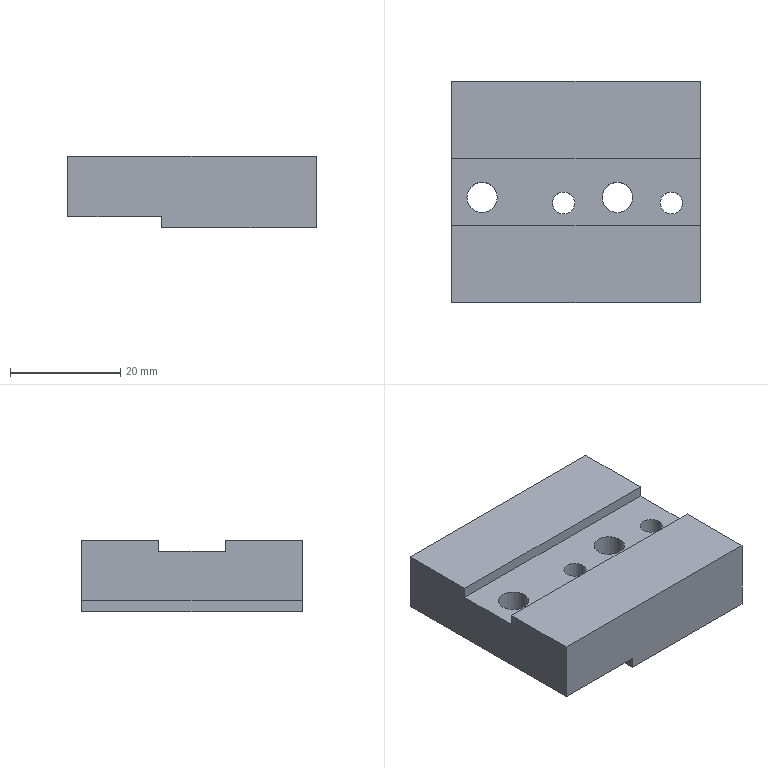Part | NX | features BREP 1 | 1 solid | 42 faces | box 45 x 40 x 13 mm | volume 19304 mm3 | cylinder 20 | plane 14 | cone 8 | commonest cylinder face diameters 3.3 x8 4 x4 5.5 x4 10 x4
STEP:
#1=CARTESIAN_POINT('',(-698.312,30.27,5.));
#2=VERTEX_POINT('',#1);
#3=CARTESIAN_POINT('',(-708.312,30.27,5.));
#4=VERTEX_POINT('',#3);
#5=CARTESIAN_POINT('',(-703.312,30.27,5.));
#6=DIRECTION('',(0.,0.,-1.));
#7=DIRECTION('',(-1.,0.,0.));
#8=AXIS2_PLACEMENT_3D('',#5,#6,#7);
#9=CIRCLE('',#8,5.);
#10=EDGE_CURVE('',#2,#4,#9,.T.);
#11=ORIENTED_EDGE('',*,*,#10,.F.);
#12=CARTESIAN_POINT('',(-698.312,30.27,0.));
#13=VERTEX_POINT('',#12);
#14=CARTESIAN_POINT('',(-698.312,30.27,0.));
#15=DIRECTION('',(0.,0.,-1.));
#16=VECTOR('',#15,1000.);
#17=LINE('',#14,#16);
#18=EDGE_CURVE('',#2,#13,#17,.T.);
#19=ORIENTED_EDGE('',*,*,#18,.T.);
#20=CARTESIAN_POINT('',(-708.312,30.27,0.));
#21=VERTEX_POINT('',#20);
#22=CARTESIAN_POINT('',(-703.312,30.27,0.));
#23=DIRECTION('',(0.,0.,-1.));
#24=DIRECTION('',(-1.,0.,0.));
#25=AXIS2_PLACEMENT_3D('',#22,#23,#24);
#26=CIRCLE('',#25,5.);
#27=EDGE_CURVE('',#13,#21,#26,.T.);
#28=ORIENTED_EDGE('',*,*,#27,.T.);
#29=CARTESIAN_POINT('',(-708.312,30.27,0.));
#30=DIRECTION('',(0.,0.,-1.));
#31=VECTOR('',#30,1000.);
#32=LINE('',#29,#31);
#33=EDGE_CURVE('',#4,#21,#32,.T.);
#34=ORIENTED_EDGE('',*,*,#33,.F.);
#35=EDGE_LOOP('',(#11,#19,#28,#34));
#36=FACE_BOUND('',#35,.T.);
#37=CARTESIAN_POINT('',(-703.312,30.27,0.));
#38=DIRECTION('',(0.,0.,-1.));
#39=DIRECTION('',(-1.,0.,0.));
#40=AXIS2_PLACEMENT_3D('',#37,#38,#39);
#41=CYLINDRICAL_SURFACE('',#40,5.);
#42=ADVANCED_FACE('',(#36),#41,.F.);
#43=CARTESIAN_POINT('',(-700.562,30.27,11.));
#44=VERTEX_POINT('',#43);
#45=CARTESIAN_POINT('',(-706.062,30.27,11.));
#46=VERTEX_POINT('',#45);
#47=CARTESIAN_POINT('',(-703.312,30.27,11.));
#48=DIRECTION('',(0.,0.,-1.));
#49=DIRECTION('',(-1.,0.,0.));
#50=AXIS2_PLACEMENT_3D('',#47,#48,#49);
#51=CIRCLE('',#50,2.75);
#52=EDGE_CURVE('',#44,#46,#51,.T.);
#53=ORIENTED_EDGE('',*,*,#52,.F.);
#54=CARTESIAN_POINT('',(-700.562,30.27,5.));
#55=VERTEX_POINT('',#54);
#56=CARTESIAN_POINT('',(-700.562,30.27,0.));
#57=DIRECTION('',(0.,0.,-1.));
#58=VECTOR('',#57,1000.);
#59=LINE('',#56,#58);
#60=EDGE_CURVE('',#44,#55,#59,.T.);
#61=ORIENTED_EDGE('',*,*,#60,.T.);
#62=CARTESIAN_POINT('',(-706.062,30.27,5.));
#63=VERTEX_POINT('',#62);
#64=CARTESIAN_POINT('',(-703.312,30.27,5.));
#65=DIRECTION('',(0.,0.,-1.));
#66=DIRECTION('',(-1.,0.,0.));
#67=AXIS2_PLACEMENT_3D('',#64,#65,#66);
#68=CIRCLE('',#67,2.75);
#69=EDGE_CURVE('',#55,#63,#68,.T.);
#70=ORIENTED_EDGE('',*,*,#69,.T.);
#71=CARTESIAN_POINT('',(-706.062,30.27,0.));
#72=DIRECTION('',(0.,0.,-1.));
#73=VECTOR('',#72,1000.);
#74=LINE('',#71,#73);
#75=EDGE_CURVE('',#46,#63,#74,.T.);
#76=ORIENTED_EDGE('',*,*,#75,.F.);
#77=EDGE_LOOP('',(#53,#61,#70,#76));
#78=FACE_BOUND('',#77,.T.);
#79=CARTESIAN_POINT('',(-703.312,30.27,0.));
#80=DIRECTION('',(0.,0.,-1.));
#81=DIRECTION('',(-1.,0.,0.));
#82=AXIS2_PLACEMENT_3D('',#79,#80,#81);
#83=CYLINDRICAL_SURFACE('',#82,2.75);
#84=ADVANCED_FACE('',(#78),#83,.F.);
#85=CARTESIAN_POINT('',(-722.812,30.27,7.));
#86=VERTEX_POINT('',#85);
#87=CARTESIAN_POINT('',(-732.812,30.27,7.));
#88=VERTEX_POINT('',#87);
#89=CARTESIAN_POINT('',(-727.812,30.27,7.));
#90=DIRECTION('',(0.,0.,-1.));
#91=DIRECTION('',(-1.,0.,0.));
#92=AXIS2_PLACEMENT_3D('',#89,#90,#91);
#93=CIRCLE('',#92,5.);
#94=EDGE_CURVE('',#86,#88,#93,.T.);
#95=ORIENTED_EDGE('',*,*,#94,.F.);
#96=CARTESIAN_POINT('',(-722.812,30.27,2.));
#97=VERTEX_POINT('',#96);
#98=CARTESIAN_POINT('',(-722.812,30.27,0.));
#99=DIRECTION('',(0.,0.,-1.));
#100=VECTOR('',#99,1000.);
#101=LINE('',#98,#100);
#102=EDGE_CURVE('',#86,#97,#101,.T.);
#103=ORIENTED_EDGE('',*,*,#102,.T.);
#104=CARTESIAN_POINT('',(-732.812,30.27,2.));
#105=VERTEX_POINT('',#104);
#106=CARTESIAN_POINT('',(-727.812,30.27,2.));
#107=DIRECTION('',(0.,0.,-1.));
#108=DIRECTION('',(1.,0.,0.));
#109=AXIS2_PLACEMENT_3D('',#106,#107,#108);
#110=CIRCLE('',#109,5.);
#111=EDGE_CURVE('',#97,#105,#110,.T.);
#112=ORIENTED_EDGE('',*,*,#111,.T.);
#113=CARTESIAN_POINT('',(-732.812,30.27,0.));
#114=DIRECTION('',(0.,0.,-1.));
#115=VECTOR('',#114,1000.);
#116=LINE('',#113,#115);
#117=EDGE_CURVE('',#88,#105,#116,.T.);
#118=ORIENTED_EDGE('',*,*,#117,.F.);
#119=EDGE_LOOP('',(#95,#103,#112,#118));
#120=FACE_BOUND('',#119,.T.);
#121=CARTESIAN_POINT('',(-727.812,30.27,0.));
#122=DIRECTION('',(0.,0.,-1.));
#123=DIRECTION('',(-1.,0.,0.));
#124=AXIS2_PLACEMENT_3D('',#121,#122,#123);
#125=CYLINDRICAL_SURFACE('',#124,5.);
#126=ADVANCED_FACE('',(#120),#125,.F.);
#127=CARTESIAN_POINT('',(-691.912,18.27,10.1));
#128=VERTEX_POINT('',#127);
#129=CARTESIAN_POINT('',(-695.212,18.27,10.1));
#130=VERTEX_POINT('',#129);
#131=CARTESIAN_POINT('',(-693.562,18.27,10.1));
#132=DIRECTION('',(0.,0.,-1.));
#133=DIRECTION('',(-1.,0.,0.));
#134=AXIS2_PLACEMENT_3D('',#131,#132,#133);
#135=CIRCLE('',#134,1.65);
#136=EDGE_CURVE('',#128,#130,#135,.T.);
#137=ORIENTED_EDGE('',*,*,#136,.F.);
#138=CARTESIAN_POINT('',(-691.912,18.27,0.));
#139=VERTEX_POINT('',#138);
#140=CARTESIAN_POINT('',(-691.912,18.27,0.));
#141=DIRECTION('',(0.,0.,-1.));
#142=VECTOR('',#141,1000.);
#143=LINE('',#140,#142);
#144=EDGE_CURVE('',#128,#139,#143,.T.);
#145=ORIENTED_EDGE('',*,*,#144,.T.);
#146=CARTESIAN_POINT('',(-695.212,18.27,0.));
#147=VERTEX_POINT('',#146);
#148=CARTESIAN_POINT('',(-693.562,18.27,0.));
#149=DIRECTION('',(0.,0.,-1.));
#150=DIRECTION('',(-1.,0.,0.));
#151=AXIS2_PLACEMENT_3D('',#148,#149,#150);
#152=CIRCLE('',#151,1.65);
#153=EDGE_CURVE('',#139,#147,#152,.T.);
#154=ORIENTED_EDGE('',*,*,#153,.T.);
#155=CARTESIAN_POINT('',(-695.212,18.27,0.));
#156=DIRECTION('',(0.,0.,-1.));
#157=VECTOR('',#156,1000.);
#158=LINE('',#155,#157);
#159=EDGE_CURVE('',#130,#147,#158,.T.);
#160=ORIENTED_EDGE('',*,*,#159,.F.);
#161=EDGE_LOOP('',(#137,#145,#154,#160));
#162=FACE_BOUND('',#161,.T.);
#163=CARTESIAN_POINT('',(-693.562,18.27,0.));
#164=DIRECTION('',(0.,0.,-1.));
#165=DIRECTION('',(-1.,0.,0.));
#166=AXIS2_PLACEMENT_3D('',#163,#164,#165);
#167=CYLINDRICAL_SURFACE('',#166,1.65);
#168=ADVANCED_FACE('',(#162),#167,.F.);
#169=CARTESIAN_POINT('',(-693.562,18.27,11.091));
#170=VERTEX_POINT('',#169);
#171=CARTESIAN_POINT('',(-695.212,18.27,10.1));
#172=DIRECTION('',(-0.8572,0.,-0.515));
#173=VECTOR('',#172,1000.);
#174=LINE('',#171,#173);
#175=EDGE_CURVE('',#170,#130,#174,.T.);
#176=ORIENTED_EDGE('',*,*,#175,.F.);
#177=CARTESIAN_POINT('',(-691.912,18.27,10.1));
#178=DIRECTION('',(0.8572,0.,-0.515));
#179=VECTOR('',#178,1000.);
#180=LINE('',#177,#179);
#181=EDGE_CURVE('',#170,#128,#180,.T.);
#182=ORIENTED_EDGE('',*,*,#181,.T.);
#183=ORIENTED_EDGE('',*,*,#136,.T.);
#184=EDGE_LOOP('',(#176,#182,#183));
#185=FACE_BOUND('',#184,.T.);
#186=CARTESIAN_POINT('',(-693.562,18.27,10.1));
#187=DIRECTION('',(0.,0.,-1.));
#188=DIRECTION('',(-1.,0.,0.));
#189=AXIS2_PLACEMENT_3D('',#186,#187,#188);
#190=CONICAL_SURFACE('',#189,1.65,1.03);
#191=ADVANCED_FACE('',(#185),#190,.F.);
#192=CARTESIAN_POINT('',(-691.912,45.27,10.1));
#193=VERTEX_POINT('',#192);
#194=CARTESIAN_POINT('',(-695.212,45.27,10.1));
#195=VERTEX_POINT('',#194);
#196=CARTESIAN_POINT('',(-693.562,45.27,10.1));
#197=DIRECTION('',(0.,0.,-1.));
#198=DIRECTION('',(-1.,0.,0.));
#199=AXIS2_PLACEMENT_3D('',#196,#197,#198);
#200=CIRCLE('',#199,1.65);
#201=EDGE_CURVE('',#193,#195,#200,.T.);
#202=ORIENTED_EDGE('',*,*,#201,.F.);
#203=CARTESIAN_POINT('',(-691.912,45.27,0.));
#204=VERTEX_POINT('',#203);
#205=CARTESIAN_POINT('',(-691.912,45.27,0.));
#206=DIRECTION('',(0.,0.,-1.));
#207=VECTOR('',#206,1000.);
#208=LINE('',#205,#207);
#209=EDGE_CURVE('',#193,#204,#208,.T.);
#210=ORIENTED_EDGE('',*,*,#209,.T.);
#211=CARTESIAN_POINT('',(-695.212,45.27,0.));
#212=VERTEX_POINT('',#211);
#213=CARTESIAN_POINT('',(-693.562,45.27,0.));
#214=DIRECTION('',(0.,0.,-1.));
#215=DIRECTION('',(-1.,0.,0.));
#216=AXIS2_PLACEMENT_3D('',#213,#214,#215);
#217=CIRCLE('',#216,1.65);
#218=EDGE_CURVE('',#204,#212,#217,.T.);
#219=ORIENTED_EDGE('',*,*,#218,.T.);
#220=CARTESIAN_POINT('',(-695.212,45.27,0.));
#221=DIRECTION('',(0.,0.,-1.));
#222=VECTOR('',#221,1000.);
#223=LINE('',#220,#222);
#224=EDGE_CURVE('',#195,#212,#223,.T.);
#225=ORIENTED_EDGE('',*,*,#224,.F.);
#226=EDGE_LOOP('',(#202,#210,#219,#225));
#227=FACE_BOUND('',#226,.T.);
#228=CARTESIAN_POINT('',(-693.562,45.27,0.));
#229=DIRECTION('',(0.,0.,-1.));
#230=DIRECTION('',(-1.,0.,0.));
#231=AXIS2_PLACEMENT_3D('',#228,#229,#230);
#232=CYLINDRICAL_SURFACE('',#231,1.65);
#233=ADVANCED_FACE('',(#227),#232,.F.);
#234=CARTESIAN_POINT('',(-693.562,45.27,11.091));
#235=VERTEX_POINT('',#234);
#236=CARTESIAN_POINT('',(-695.212,45.27,10.1));
#237=DIRECTION('',(-0.8572,0.,-0.515));
#238=VECTOR('',#237,1000.);
#239=LINE('',#236,#238);
#240=EDGE_CURVE('',#235,#195,#239,.T.);
#241=ORIENTED_EDGE('',*,*,#240,.F.);
#242=CARTESIAN_POINT('',(-691.912,45.27,10.1));
#243=DIRECTION('',(0.8572,0.,-0.515));
#244=VECTOR('',#243,1000.);
#245=LINE('',#242,#244);
#246=EDGE_CURVE('',#235,#193,#245,.T.);
#247=ORIENTED_EDGE('',*,*,#246,.T.);
#248=ORIENTED_EDGE('',*,*,#201,.T.);
#249=EDGE_LOOP('',(#241,#247,#248));
#250=FACE_BOUND('',#249,.T.);
#251=CARTESIAN_POINT('',(-693.562,45.27,10.1));
#252=DIRECTION('',(0.,0.,-1.));
#253=DIRECTION('',(-1.,0.,0.));
#254=AXIS2_PLACEMENT_3D('',#251,#252,#253);
#255=CONICAL_SURFACE('',#254,1.65,1.03);
#256=ADVANCED_FACE('',(#250),#255,.F.);
#257=CARTESIAN_POINT('',(-711.412,45.27,10.1));
#258=VERTEX_POINT('',#257);
#259=CARTESIAN_POINT('',(-714.712,45.27,10.1));
#260=VERTEX_POINT('',#259);
#261=CARTESIAN_POINT('',(-713.062,45.27,10.1));
#262=DIRECTION('',(0.,0.,-1.));
#263=DIRECTION('',(-1.,0.,0.));
#264=AXIS2_PLACEMENT_3D('',#261,#262,#263);
#265=CIRCLE('',#264,1.65);
#266=EDGE_CURVE('',#258,#260,#265,.T.);
#267=ORIENTED_EDGE('',*,*,#266,.F.);
#268=CARTESIAN_POINT('',(-711.412,45.27,0.));
#269=VERTEX_POINT('',#268);
#270=CARTESIAN_POINT('',(-711.412,45.27,0.));
#271=DIRECTION('',(0.,0.,-1.));
#272=VECTOR('',#271,1000.);
#273=LINE('',#270,#272);
#274=EDGE_CURVE('',#258,#269,#273,.T.);
#275=ORIENTED_EDGE('',*,*,#274,.T.);
#276=CARTESIAN_POINT('',(-714.712,45.27,0.));
#277=VERTEX_POINT('',#276);
#278=CARTESIAN_POINT('',(-713.062,45.27,0.));
#279=DIRECTION('',(0.,0.,-1.));
#280=DIRECTION('',(-1.,0.,0.));
#281=AXIS2_PLACEMENT_3D('',#278,#279,#280);
#282=CIRCLE('',#281,1.65);
#283=EDGE_CURVE('',#269,#277,#282,.T.);
#284=ORIENTED_EDGE('',*,*,#283,.T.);
#285=CARTESIAN_POINT('',(-714.712,45.27,0.));
#286=DIRECTION('',(0.,0.,-1.));
#287=VECTOR('',#286,1000.);
#288=LINE('',#285,#287);
#289=EDGE_CURVE('',#260,#277,#288,.T.);
#290=ORIENTED_EDGE('',*,*,#289,.F.);
#291=EDGE_LOOP('',(#267,#275,#284,#290));
#292=FACE_BOUND('',#291,.T.);
#293=CARTESIAN_POINT('',(-713.062,45.27,0.));
#294=DIRECTION('',(0.,0.,-1.));
#295=DIRECTION('',(-1.,0.,0.));
#296=AXIS2_PLACEMENT_3D('',#293,#294,#295);
#297=CYLINDRICAL_SURFACE('',#296,1.65);
#298=ADVANCED_FACE('',(#292),#297,.F.);
#299=CARTESIAN_POINT('',(-713.062,45.27,11.091));
#300=VERTEX_POINT('',#299);
#301=CARTESIAN_POINT('',(-714.712,45.27,10.1));
#302=DIRECTION('',(-0.8572,0.,-0.515));
#303=VECTOR('',#302,1000.);
#304=LINE('',#301,#303);
#305=EDGE_CURVE('',#300,#260,#304,.T.);
#306=ORIENTED_EDGE('',*,*,#305,.F.);
#307=CARTESIAN_POINT('',(-711.412,45.27,10.1));
#308=DIRECTION('',(0.8572,0.,-0.515));
#309=VECTOR('',#308,1000.);
#310=LINE('',#307,#309);
#311=EDGE_CURVE('',#300,#258,#310,.T.);
#312=ORIENTED_EDGE('',*,*,#311,.T.);
#313=ORIENTED_EDGE('',*,*,#266,.T.);
#314=EDGE_LOOP('',(#306,#312,#313));
#315=FACE_BOUND('',#314,.T.);
#316=CARTESIAN_POINT('',(-713.062,45.27,10.1));
#317=DIRECTION('',(0.,0.,-1.));
#318=DIRECTION('',(-1.,0.,0.));
#319=AXIS2_PLACEMENT_3D('',#316,#317,#318);
#320=CONICAL_SURFACE('',#319,1.65,1.03);
#321=ADVANCED_FACE('',(#315),#320,.F.);
#322=CARTESIAN_POINT('',(-711.412,18.27,10.1));
#323=VERTEX_POINT('',#322);
#324=CARTESIAN_POINT('',(-714.712,18.27,10.1));
#325=VERTEX_POINT('',#324);
#326=CARTESIAN_POINT('',(-713.062,18.27,10.1));
#327=DIRECTION('',(0.,0.,-1.));
#328=DIRECTION('',(-1.,0.,0.));
#329=AXIS2_PLACEMENT_3D('',#326,#327,#328);
#330=CIRCLE('',#329,1.65);
#331=EDGE_CURVE('',#323,#325,#330,.T.);
#332=ORIENTED_EDGE('',*,*,#331,.F.);
#333=CARTESIAN_POINT('',(-711.412,18.27,0.));
#334=VERTEX_POINT('',#333);
#335=CARTESIAN_POINT('',(-711.412,18.27,0.));
#336=DIRECTION('',(0.,0.,-1.));
#337=VECTOR('',#336,1000.);
#338=LINE('',#335,#337);
#339=EDGE_CURVE('',#323,#334,#338,.T.);
#340=ORIENTED_EDGE('',*,*,#339,.T.);
#341=CARTESIAN_POINT('',(-714.712,18.27,0.));
#342=VERTEX_POINT('',#341);
#343=CARTESIAN_POINT('',(-713.062,18.27,0.));
#344=DIRECTION('',(0.,0.,-1.));
#345=DIRECTION('',(-1.,0.,0.));
#346=AXIS2_PLACEMENT_3D('',#343,#344,#345);
#347=CIRCLE('',#346,1.65);
#348=EDGE_CURVE('',#334,#342,#347,.T.);
#349=ORIENTED_EDGE('',*,*,#348,.T.);
#350=CARTESIAN_POINT('',(-714.712,18.27,0.));
#351=DIRECTION('',(0.,0.,-1.));
#352=VECTOR('',#351,1000.);
#353=LINE('',#350,#352);
#354=EDGE_CURVE('',#325,#342,#353,.T.);
#355=ORIENTED_EDGE('',*,*,#354,.F.);
#356=EDGE_LOOP('',(#332,#340,#349,#355));
#357=FACE_BOUND('',#356,.T.);
#358=CARTESIAN_POINT('',(-713.062,18.27,0.));
#359=DIRECTION('',(0.,0.,-1.));
#360=DIRECTION('',(-1.,0.,0.));
#361=AXIS2_PLACEMENT_3D('',#358,#359,#360);
#362=CYLINDRICAL_SURFACE('',#361,1.65);
#363=ADVANCED_FACE('',(#357),#362,.F.);
#364=CARTESIAN_POINT('',(-713.062,18.27,11.091));
#365=VERTEX_POINT('',#364);
#366=CARTESIAN_POINT('',(-714.712,18.27,10.1));
#367=DIRECTION('',(-0.8572,0.,-0.515));
#368=VECTOR('',#367,1000.);
#369=LINE('',#366,#368);
#370=EDGE_CURVE('',#365,#325,#369,.T.);
#371=ORIENTED_EDGE('',*,*,#370,.F.);
#372=CARTESIAN_POINT('',(-711.412,18.27,10.1));
#373=DIRECTION('',(0.8572,0.,-0.515));
#374=VECTOR('',#373,1000.);
#375=LINE('',#372,#374);
#376=EDGE_CURVE('',#365,#323,#375,.T.);
#377=ORIENTED_EDGE('',*,*,#376,.T.);
#378=ORIENTED_EDGE('',*,*,#331,.T.);
#379=EDGE_LOOP('',(#371,#377,#378));
#380=FACE_BOUND('',#379,.T.);
#381=CARTESIAN_POINT('',(-713.062,18.27,10.1));
#382=DIRECTION('',(0.,0.,-1.));
#383=DIRECTION('',(-1.,0.,0.));
#384=AXIS2_PLACEMENT_3D('',#381,#382,#383);
#385=CONICAL_SURFACE('',#384,1.65,1.03);
#386=ADVANCED_FACE('',(#380),#385,.F.);
#387=CARTESIAN_POINT('',(-711.062,29.27,11.));
#388=VERTEX_POINT('',#387);
#389=CARTESIAN_POINT('',(-715.062,29.27,11.));
#390=VERTEX_POINT('',#389);
#391=CARTESIAN_POINT('',(-713.062,29.27,11.));
#392=DIRECTION('',(0.,0.,-1.));
#393=DIRECTION('',(-1.,0.,0.));
#394=AXIS2_PLACEMENT_3D('',#391,#392,#393);
#395=CIRCLE('',#394,2.);
#396=EDGE_CURVE('',#388,#390,#395,.T.);
#397=ORIENTED_EDGE('',*,*,#396,.F.);
#398=CARTESIAN_POINT('',(-711.062,29.27,0.));
#399=VERTEX_POINT('',#398);
#400=CARTESIAN_POINT('',(-711.062,29.27,13.));
#401=DIRECTION('',(0.,0.,-1.));
#402=VECTOR('',#401,1000.);
#403=LINE('',#400,#402);
#404=EDGE_CURVE('',#388,#399,#403,.T.);
#405=ORIENTED_EDGE('',*,*,#404,.T.);
#406=CARTESIAN_POINT('',(-715.062,29.27,0.));
#407=VERTEX_POINT('',#406);
#408=CARTESIAN_POINT('',(-713.062,29.27,0.));
#409=DIRECTION('',(0.,0.,-1.));
#410=DIRECTION('',(-1.,0.,0.));
#411=AXIS2_PLACEMENT_3D('',#408,#409,#410);
#412=CIRCLE('',#411,2.);
#413=EDGE_CURVE('',#399,#407,#412,.T.);
#414=ORIENTED_EDGE('',*,*,#413,.T.);
#415=CARTESIAN_POINT('',(-715.062,29.27,13.));
#416=DIRECTION('',(0.,0.,-1.));
#417=VECTOR('',#416,1000.);
#418=LINE('',#415,#417);
#419=EDGE_CURVE('',#390,#407,#418,.T.);
#420=ORIENTED_EDGE('',*,*,#419,.F.);
#421=EDGE_LOOP('',(#397,#405,#414,#420));
#422=FACE_BOUND('',#421,.T.);
#423=CARTESIAN_POINT('',(-713.062,29.27,13.));
#424=DIRECTION('',(0.,0.,-1.));
#425=DIRECTION('',(-1.,0.,0.));
#426=AXIS2_PLACEMENT_3D('',#423,#424,#425);
#427=CYLINDRICAL_SURFACE('',#426,2.);
#428=ADVANCED_FACE('',(#422),#427,.F.);
#429=CARTESIAN_POINT('',(-691.562,29.27,11.));
#430=VERTEX_POINT('',#429);
#431=CARTESIAN_POINT('',(-695.562,29.27,11.));
#432=VERTEX_POINT('',#431);
#433=CARTESIAN_POINT('',(-693.562,29.27,11.));
#434=DIRECTION('',(0.,0.,-1.));
#435=DIRECTION('',(-1.,0.,0.));
#436=AXIS2_PLACEMENT_3D('',#433,#434,#435);
#437=CIRCLE('',#436,2.);
#438=EDGE_CURVE('',#430,#432,#437,.T.);
#439=ORIENTED_EDGE('',*,*,#438,.F.);
#440=CARTESIAN_POINT('',(-691.562,29.27,0.));
#441=VERTEX_POINT('',#440);
#442=CARTESIAN_POINT('',(-691.562,29.27,13.));
#443=DIRECTION('',(0.,0.,-1.));
#444=VECTOR('',#443,1000.);
#445=LINE('',#442,#444);
#446=EDGE_CURVE('',#430,#441,#445,.T.);
#447=ORIENTED_EDGE('',*,*,#446,.T.);
#448=CARTESIAN_POINT('',(-695.562,29.27,0.));
#449=VERTEX_POINT('',#448);
#450=CARTESIAN_POINT('',(-693.562,29.27,0.));
#451=DIRECTION('',(0.,0.,-1.));
#452=DIRECTION('',(-1.,0.,0.));
#453=AXIS2_PLACEMENT_3D('',#450,#451,#452);
#454=CIRCLE('',#453,2.);
#455=EDGE_CURVE('',#441,#449,#454,.T.);
#456=ORIENTED_EDGE('',*,*,#455,.T.);
#457=CARTESIAN_POINT('',(-695.562,29.27,13.));
#458=DIRECTION('',(0.,0.,-1.));
#459=VECTOR('',#458,1000.);
#460=LINE('',#457,#459);
#461=EDGE_CURVE('',#432,#449,#460,.T.);
#462=ORIENTED_EDGE('',*,*,#461,.F.);
#463=EDGE_LOOP('',(#439,#447,#456,#462));
#464=FACE_BOUND('',#463,.T.);
#465=CARTESIAN_POINT('',(-693.562,29.27,13.));
#466=DIRECTION('',(0.,0.,-1.));
#467=DIRECTION('',(-1.,0.,0.));
#468=AXIS2_PLACEMENT_3D('',#465,#466,#467);
#469=CYLINDRICAL_SURFACE('',#468,2.);
#470=ADVANCED_FACE('',(#464),#469,.F.);
#471=CARTESIAN_POINT('',(-725.062,30.27,11.));
#472=VERTEX_POINT('',#471);
#473=CARTESIAN_POINT('',(-730.562,30.27,11.));
#474=VERTEX_POINT('',#473);
#475=CARTESIAN_POINT('',(-727.812,30.27,11.));
#476=DIRECTION('',(0.,0.,-1.));
#477=DIRECTION('',(-1.,0.,0.));
#478=AXIS2_PLACEMENT_3D('',#475,#476,#477);
#479=CIRCLE('',#478,2.75);
#480=EDGE_CURVE('',#472,#474,#479,.T.);
#481=ORIENTED_EDGE('',*,*,#480,.F.);
#482=CARTESIAN_POINT('',(-725.062,30.27,7.));
#483=VERTEX_POINT('',#482);
#484=CARTESIAN_POINT('',(-725.062,30.27,0.));
#485=DIRECTION('',(0.,0.,-1.));
#486=VECTOR('',#485,1000.);
#487=LINE('',#484,#486);
#488=EDGE_CURVE('',#472,#483,#487,.T.);
#489=ORIENTED_EDGE('',*,*,#488,.T.);
#490=CARTESIAN_POINT('',(-730.562,30.27,7.));
#491=VERTEX_POINT('',#490);
#492=CARTESIAN_POINT('',(-727.812,30.27,7.));
#493=DIRECTION('',(0.,0.,1.));
#494=DIRECTION('',(-1.,0.,0.));
#495=AXIS2_PLACEMENT_3D('',#492,#493,#494);
#496=CIRCLE('',#495,2.75);
#497=EDGE_CURVE('',#491,#483,#496,.T.);
#498=ORIENTED_EDGE('',*,*,#497,.F.);
#499=CARTESIAN_POINT('',(-730.562,30.27,0.));
#500=DIRECTION('',(0.,0.,-1.));
#501=VECTOR('',#500,1000.);
#502=LINE('',#499,#501);
#503=EDGE_CURVE('',#474,#491,#502,.T.);
#504=ORIENTED_EDGE('',*,*,#503,.F.);
#505=EDGE_LOOP('',(#481,#489,#498,#504));
#506=FACE_BOUND('',#505,.T.);
#507=CARTESIAN_POINT('',(-727.812,30.27,0.));
#508=DIRECTION('',(0.,0.,-1.));
#509=DIRECTION('',(-1.,0.,0.));
#510=AXIS2_PLACEMENT_3D('',#507,#508,#509);
#511=CYLINDRICAL_SURFACE('',#510,2.75);
#512=ADVANCED_FACE('',(#506),#511,.F.);
#513=ORIENTED_EDGE('',*,*,#488,.F.);
#514=CARTESIAN_POINT('',(-727.812,30.27,11.));
#515=DIRECTION('',(0.,0.,-1.));
#516=DIRECTION('',(-1.,0.,0.));
#517=AXIS2_PLACEMENT_3D('',#514,#515,#516);
#518=CIRCLE('',#517,2.75);
#519=EDGE_CURVE('',#474,#472,#518,.T.);
#520=ORIENTED_EDGE('',*,*,#519,.F.);
#521=ORIENTED_EDGE('',*,*,#503,.T.);
#522=CARTESIAN_POINT('',(-727.812,30.27,7.));
#523=DIRECTION('',(0.,0.,1.));
#524=DIRECTION('',(-1.,0.,0.));
#525=AXIS2_PLACEMENT_3D('',#522,#523,#524);
#526=CIRCLE('',#525,2.75);
#527=EDGE_CURVE('',#483,#491,#526,.T.);
#528=ORIENTED_EDGE('',*,*,#527,.F.);
#529=EDGE_LOOP('',(#513,#520,#521,#528));
#530=FACE_BOUND('',#529,.T.);
#531=CARTESIAN_POINT('',(-727.812,30.27,0.));
#532=DIRECTION('',(0.,0.,-1.));
#533=DIRECTION('',(-1.,0.,0.));
#534=AXIS2_PLACEMENT_3D('',#531,#532,#533);
#535=CYLINDRICAL_SURFACE('',#534,2.75);
#536=ADVANCED_FACE('',(#530),#535,.F.);
#537=CARTESIAN_POINT('',(-688.312,25.27,13.));
#538=VERTEX_POINT('',#537);
#539=CARTESIAN_POINT('',(-733.312,25.27,13.));
#540=VERTEX_POINT('',#539);
#541=CARTESIAN_POINT('',(-688.312,25.27,13.));
#542=DIRECTION('',(-1.,0.,0.));
#543=VECTOR('',#542,1000.);
#544=LINE('',#541,#543);
#545=EDGE_CURVE('',#538,#540,#544,.T.);
#546=ORIENTED_EDGE('',*,*,#545,.T.);
#547=CARTESIAN_POINT('',(-733.312,11.27,13.));
#548=VERTEX_POINT('',#547);
#549=CARTESIAN_POINT('',(-733.312,51.27,13.));
#550=DIRECTION('',(0.,-1.,0.));
#551=VECTOR('',#550,1000.);
#552=LINE('',#549,#551);
#553=EDGE_CURVE('',#540,#548,#552,.T.);
#554=ORIENTED_EDGE('',*,*,#553,.T.);
#555=CARTESIAN_POINT('',(-688.312,11.27,13.));
#556=VERTEX_POINT('',#555);
#557=CARTESIAN_POINT('',(-743.312,11.27,13.));
#558=DIRECTION('',(1.,0.,0.));
#559=VECTOR('',#558,1000.);
#560=LINE('',#557,#559);
#561=EDGE_CURVE('',#548,#556,#560,.T.);
#562=ORIENTED_EDGE('',*,*,#561,.T.);
#563=CARTESIAN_POINT('',(-688.312,11.27,13.));
#564=DIRECTION('',(0.,1.,0.));
#565=VECTOR('',#564,1000.);
#566=LINE('',#563,#565);
#567=EDGE_CURVE('',#556,#538,#566,.T.);
#568=ORIENTED_EDGE('',*,*,#567,.T.);
#569=EDGE_LOOP('',(#546,#554,#562,#568));
#570=FACE_BOUND('',#569,.T.);
#571=CARTESIAN_POINT('',(-743.312,51.27,13.));
#572=DIRECTION('',(0.,0.,-1.));
#573=DIRECTION('',(0.,-1.,0.));
#574=AXIS2_PLACEMENT_3D('',#571,#572,#573);
#575=PLANE('',#574);
#576=ADVANCED_FACE('',(#570),#575,.F.);
#577=CARTESIAN_POINT('',(-733.312,11.27,2.));
#578=VERTEX_POINT('',#577);
#579=CARTESIAN_POINT('',(-733.312,11.27,13.));
#580=DIRECTION('',(0.,0.,-1.));
#581=VECTOR('',#580,1000.);
#582=LINE('',#579,#581);
#583=EDGE_CURVE('',#548,#578,#582,.T.);
#584=ORIENTED_EDGE('',*,*,#583,.T.);
#585=CARTESIAN_POINT('',(-716.312,11.27,2.));
#586=VERTEX_POINT('',#585);
#587=CARTESIAN_POINT('',(-733.312,11.27,2.));
#588=DIRECTION('',(-1.,0.,0.));
#589=VECTOR('',#588,1000.);
#590=LINE('',#587,#589);
#591=EDGE_CURVE('',#586,#578,#590,.T.);
#592=ORIENTED_EDGE('',*,*,#591,.F.);
#593=CARTESIAN_POINT('',(-716.312,11.27,0.));
#594=VERTEX_POINT('',#593);
#595=CARTESIAN_POINT('',(-716.312,11.27,0.));
#596=DIRECTION('',(0.,0.,1.));
#597=VECTOR('',#596,1000.);
#598=LINE('',#595,#597);
#599=EDGE_CURVE('',#594,#586,#598,.T.);
#600=ORIENTED_EDGE('',*,*,#599,.F.);
#601=CARTESIAN_POINT('',(-688.312,11.27,0.));
#602=VERTEX_POINT('',#601);
#603=CARTESIAN_POINT('',(-743.312,11.27,0.));
#604=DIRECTION('',(1.,0.,0.));
#605=VECTOR('',#604,1000.);
#606=LINE('',#603,#605);
#607=EDGE_CURVE('',#594,#602,#606,.T.);
#608=ORIENTED_EDGE('',*,*,#607,.T.);
#609=CARTESIAN_POINT('',(-688.312,11.27,13.));
#610=DIRECTION('',(0.,0.,-1.));
#611=VECTOR('',#610,1000.);
#612=LINE('',#609,#611);
#613=EDGE_CURVE('',#556,#602,#612,.T.);
#614=ORIENTED_EDGE('',*,*,#613,.F.);
#615=ORIENTED_EDGE('',*,*,#561,.F.);
#616=EDGE_LOOP('',(#584,#592,#600,#608,#614,#615));
#617=FACE_BOUND('',#616,.T.);
#618=CARTESIAN_POINT('',(-743.312,11.27,13.));
#619=DIRECTION('',(0.,1.,0.));
#620=DIRECTION('',(1.,0.,0.));
#621=AXIS2_PLACEMENT_3D('',#618,#619,#620);
#622=PLANE('',#621);
#623=ADVANCED_FACE('',(#617),#622,.F.);
#624=CARTESIAN_POINT('',(-688.312,37.27,11.));
#625=VERTEX_POINT('',#624);
#626=CARTESIAN_POINT('',(-688.312,25.27,11.));
#627=VERTEX_POINT('',#626);
#628=CARTESIAN_POINT('',(-688.312,25.27,11.));
#629=DIRECTION('',(0.,-1.,0.));
#630=VECTOR('',#629,1000.);
#631=LINE('',#628,#630);
#632=EDGE_CURVE('',#625,#627,#631,.T.);
#633=ORIENTED_EDGE('',*,*,#632,.T.);
#634=CARTESIAN_POINT('',(-688.312,25.27,13.));
#635=DIRECTION('',(0.,0.,1.));
#636=VECTOR('',#635,1000.);
#637=LINE('',#634,#636);
#638=EDGE_CURVE('',#627,#538,#637,.T.);
#639=ORIENTED_EDGE('',*,*,#638,.T.);
#640=ORIENTED_EDGE('',*,*,#567,.F.);
#641=ORIENTED_EDGE('',*,*,#613,.T.);
#642=CARTESIAN_POINT('',(-688.312,51.27,0.));
#643=VERTEX_POINT('',#642);
#644=CARTESIAN_POINT('',(-688.312,11.27,0.));
#645=DIRECTION('',(0.,1.,0.));
#646=VECTOR('',#645,1000.);
#647=LINE('',#644,#646);
#648=EDGE_CURVE('',#602,#643,#647,.T.);
#649=ORIENTED_EDGE('',*,*,#648,.T.);
#650=CARTESIAN_POINT('',(-688.312,51.27,13.));
#651=VERTEX_POINT('',#650);
#652=CARTESIAN_POINT('',(-688.312,51.27,13.));
#653=DIRECTION('',(0.,0.,-1.));
#654=VECTOR('',#653,1000.);
#655=LINE('',#652,#654);
#656=EDGE_CURVE('',#651,#643,#655,.T.);
#657=ORIENTED_EDGE('',*,*,#656,.F.);
#658=CARTESIAN_POINT('',(-688.312,37.27,13.));
#659=VERTEX_POINT('',#658);
#660=CARTESIAN_POINT('',(-688.312,11.27,13.));
#661=DIRECTION('',(0.,1.,0.));
#662=VECTOR('',#661,1000.);
#663=LINE('',#660,#662);
#664=EDGE_CURVE('',#659,#651,#663,.T.);
#665=ORIENTED_EDGE('',*,*,#664,.F.);
#666=CARTESIAN_POINT('',(-688.312,37.27,13.));
#667=DIRECTION('',(0.,0.,-1.));
#668=VECTOR('',#667,1000.);
#669=LINE('',#666,#668);
#670=EDGE_CURVE('',#659,#625,#669,.T.);
#671=ORIENTED_EDGE('',*,*,#670,.T.);
#672=EDGE_LOOP('',(#633,#639,#640,#641,#649,#657,#665,#671));
#673=FACE_BOUND('',#672,.T.);
#674=CARTESIAN_POINT('',(-688.312,11.27,13.));
#675=DIRECTION('',(-1.,0.,0.));
#676=DIRECTION('',(0.,0.,1.));
#677=AXIS2_PLACEMENT_3D('',#674,#675,#676);
#678=PLANE('',#677);
#679=ADVANCED_FACE('',(#673),#678,.F.);
#680=CARTESIAN_POINT('',(-716.312,51.27,0.));
#681=VERTEX_POINT('',#680);
#682=CARTESIAN_POINT('',(-716.312,51.27,2.));
#683=VERTEX_POINT('',#682);
#684=CARTESIAN_POINT('',(-716.312,51.27,0.));
#685=DIRECTION('',(0.,0.,1.));
#686=VECTOR('',#685,1000.);
#687=LINE('',#684,#686);
#688=EDGE_CURVE('',#681,#683,#687,.T.);
#689=ORIENTED_EDGE('',*,*,#688,.T.);
#690=CARTESIAN_POINT('',(-733.312,51.27,2.));
#691=VERTEX_POINT('',#690);
#692=CARTESIAN_POINT('',(-733.312,51.27,2.));
#693=DIRECTION('',(-1.,0.,0.));
#694=VECTOR('',#693,1000.);
#695=LINE('',#692,#694);
#696=EDGE_CURVE('',#683,#691,#695,.T.);
#697=ORIENTED_EDGE('',*,*,#696,.T.);
#698=CARTESIAN_POINT('',(-733.312,51.27,13.));
#699=VERTEX_POINT('',#698);
#700=CARTESIAN_POINT('',(-733.312,51.27,13.));
#701=DIRECTION('',(0.,0.,-1.));
#702=VECTOR('',#701,1000.);
#703=LINE('',#700,#702);
#704=EDGE_CURVE('',#699,#691,#703,.T.);
#705=ORIENTED_EDGE('',*,*,#704,.F.);
#706=CARTESIAN_POINT('',(-743.312,51.27,13.));
#707=DIRECTION('',(-1.,0.,0.));
#708=VECTOR('',#707,1000.);
#709=LINE('',#706,#708);
#710=EDGE_CURVE('',#651,#699,#709,.T.);
#711=ORIENTED_EDGE('',*,*,#710,.F.);
#712=ORIENTED_EDGE('',*,*,#656,.T.);
#713=CARTESIAN_POINT('',(-743.312,51.27,0.));
#714=DIRECTION('',(-1.,0.,0.));
#715=VECTOR('',#714,1000.);
#716=LINE('',#713,#715);
#717=EDGE_CURVE('',#643,#681,#716,.T.);
#718=ORIENTED_EDGE('',*,*,#717,.T.);
#719=EDGE_LOOP('',(#689,#697,#705,#711,#712,#718));
#720=FACE_BOUND('',#719,.T.);
#721=CARTESIAN_POINT('',(-743.312,51.27,13.));
#722=DIRECTION('',(0.,-1.,0.));
#723=DIRECTION('',(0.,0.,-1.));
#724=AXIS2_PLACEMENT_3D('',#721,#722,#723);
#725=PLANE('',#724);
#726=ADVANCED_FACE('',(#720),#725,.F.);
#727=ORIENTED_EDGE('',*,*,#710,.T.);
#728=CARTESIAN_POINT('',(-733.312,37.27,13.));
#729=VERTEX_POINT('',#728);
#730=CARTESIAN_POINT('',(-733.312,51.27,13.));
#731=DIRECTION('',(0.,-1.,0.));
#732=VECTOR('',#731,1000.);
#733=LINE('',#730,#732);
#734=EDGE_CURVE('',#699,#729,#733,.T.);
#735=ORIENTED_EDGE('',*,*,#734,.T.);
#736=CARTESIAN_POINT('',(-688.312,37.27,13.));
#737=DIRECTION('',(-1.,0.,0.));
#738=VECTOR('',#737,1000.);
#739=LINE('',#736,#738);
#740=EDGE_CURVE('',#659,#729,#739,.T.);
#741=ORIENTED_EDGE('',*,*,#740,.F.);
#742=ORIENTED_EDGE('',*,*,#664,.T.);
#743=EDGE_LOOP('',(#727,#735,#741,#742));
#744=FACE_BOUND('',#743,.T.);
#745=CARTESIAN_POINT('',(-743.312,51.27,13.));
#746=DIRECTION('',(0.,0.,-1.));
#747=DIRECTION('',(0.,-1.,0.));
#748=AXIS2_PLACEMENT_3D('',#745,#746,#747);
#749=PLANE('',#748);
#750=ADVANCED_FACE('',(#744),#749,.F.);
#751=CARTESIAN_POINT('',(-716.312,51.27,0.));
#752=DIRECTION('',(0.,-1.,0.));
#753=VECTOR('',#752,1000.);
#754=LINE('',#751,#753);
#755=EDGE_CURVE('',#681,#594,#754,.T.);
#756=ORIENTED_EDGE('',*,*,#755,.F.);
#757=ORIENTED_EDGE('',*,*,#717,.F.);
#758=ORIENTED_EDGE('',*,*,#648,.F.);
#759=ORIENTED_EDGE('',*,*,#607,.F.);
#760=EDGE_LOOP('',(#756,#757,#758,#759));
#761=FACE_BOUND('',#760,.T.);
#762=CARTESIAN_POINT('',(-703.312,30.27,0.));
#763=DIRECTION('',(0.,0.,-1.));
#764=DIRECTION('',(-1.,0.,0.));
#765=AXIS2_PLACEMENT_3D('',#762,#763,#764);
#766=CIRCLE('',#765,5.);
#767=EDGE_CURVE('',#21,#13,#766,.T.);
#768=ORIENTED_EDGE('',*,*,#767,.F.);
#769=ORIENTED_EDGE('',*,*,#27,.F.);
#770=EDGE_LOOP('',(#768,#769));
#771=FACE_BOUND('',#770,.T.);
#772=CARTESIAN_POINT('',(-693.562,18.27,0.));
#773=DIRECTION('',(0.,0.,-1.));
#774=DIRECTION('',(-1.,0.,0.));
#775=AXIS2_PLACEMENT_3D('',#772,#773,#774);
#776=CIRCLE('',#775,1.65);
#777=EDGE_CURVE('',#147,#139,#776,.T.);
#778=ORIENTED_EDGE('',*,*,#777,.F.);
#779=ORIENTED_EDGE('',*,*,#153,.F.);
#780=EDGE_LOOP('',(#778,#779));
#781=FACE_BOUND('',#780,.T.);
#782=CARTESIAN_POINT('',(-693.562,45.27,0.));
#783=DIRECTION('',(0.,0.,-1.));
#784=DIRECTION('',(-1.,0.,0.));
#785=AXIS2_PLACEMENT_3D('',#782,#783,#784);
#786=CIRCLE('',#785,1.65);
#787=EDGE_CURVE('',#212,#204,#786,.T.);
#788=ORIENTED_EDGE('',*,*,#787,.F.);
#789=ORIENTED_EDGE('',*,*,#218,.F.);
#790=EDGE_LOOP('',(#788,#789));
#791=FACE_BOUND('',#790,.T.);
#792=CARTESIAN_POINT('',(-713.062,45.27,0.));
#793=DIRECTION('',(0.,0.,-1.));
#794=DIRECTION('',(-1.,0.,0.));
#795=AXIS2_PLACEMENT_3D('',#792,#793,#794);
#796=CIRCLE('',#795,1.65);
#797=EDGE_CURVE('',#277,#269,#796,.T.);
#798=ORIENTED_EDGE('',*,*,#797,.F.);
#799=ORIENTED_EDGE('',*,*,#283,.F.);
#800=EDGE_LOOP('',(#798,#799));
#801=FACE_BOUND('',#800,.T.);
#802=CARTESIAN_POINT('',(-713.062,18.27,0.));
#803=DIRECTION('',(0.,0.,-1.));
#804=DIRECTION('',(-1.,0.,0.));
#805=AXIS2_PLACEMENT_3D('',#802,#803,#804);
#806=CIRCLE('',#805,1.65);
#807=EDGE_CURVE('',#342,#334,#806,.T.);
#808=ORIENTED_EDGE('',*,*,#807,.F.);
#809=ORIENTED_EDGE('',*,*,#348,.F.);
#810=EDGE_LOOP('',(#808,#809));
#811=FACE_BOUND('',#810,.T.);
#812=CARTESIAN_POINT('',(-713.062,29.27,0.));
#813=DIRECTION('',(0.,0.,-1.));
#814=DIRECTION('',(-1.,0.,0.));
#815=AXIS2_PLACEMENT_3D('',#812,#813,#814);
#816=CIRCLE('',#815,2.);
#817=EDGE_CURVE('',#407,#399,#816,.T.);
#818=ORIENTED_EDGE('',*,*,#817,.F.);
#819=ORIENTED_EDGE('',*,*,#413,.F.);
#820=EDGE_LOOP('',(#818,#819));
#821=FACE_BOUND('',#820,.T.);
#822=CARTESIAN_POINT('',(-693.562,29.27,0.));
#823=DIRECTION('',(0.,0.,-1.));
#824=DIRECTION('',(-1.,0.,0.));
#825=AXIS2_PLACEMENT_3D('',#822,#823,#824);
#826=CIRCLE('',#825,2.);
#827=EDGE_CURVE('',#449,#441,#826,.T.);
#828=ORIENTED_EDGE('',*,*,#827,.F.);
#829=ORIENTED_EDGE('',*,*,#455,.F.);
#830=EDGE_LOOP('',(#828,#829));
#831=FACE_BOUND('',#830,.T.);
#832=CARTESIAN_POINT('',(-743.312,51.27,0.));
#833=DIRECTION('',(0.,0.,-1.));
#834=DIRECTION('',(0.,-1.,0.));
#835=AXIS2_PLACEMENT_3D('',#832,#833,#834);
#836=PLANE('',#835);
#837=ADVANCED_FACE('',(#761,#771,#781,#791,#801,#811,#821,#831),#836,.T.);
#838=CARTESIAN_POINT('',(-733.312,25.27,11.));
#839=VERTEX_POINT('',#838);
#840=CARTESIAN_POINT('',(-688.312,25.27,11.));
#841=DIRECTION('',(-1.,0.,0.));
#842=VECTOR('',#841,1000.);
#843=LINE('',#840,#842);
#844=EDGE_CURVE('',#627,#839,#843,.T.);
#845=ORIENTED_EDGE('',*,*,#844,.T.);
#846=CARTESIAN_POINT('',(-733.312,25.27,13.));
#847=DIRECTION('',(0.,0.,1.));
#848=VECTOR('',#847,1000.);
#849=LINE('',#846,#848);
#850=EDGE_CURVE('',#839,#540,#849,.T.);
#851=ORIENTED_EDGE('',*,*,#850,.T.);
#852=ORIENTED_EDGE('',*,*,#545,.F.);
#853=ORIENTED_EDGE('',*,*,#638,.F.);
#854=EDGE_LOOP('',(#845,#851,#852,#853));
#855=FACE_BOUND('',#854,.T.);
#856=CARTESIAN_POINT('',(-688.312,25.27,13.));
#857=DIRECTION('',(0.,-1.,0.));
#858=DIRECTION('',(0.,0.,-1.));
#859=AXIS2_PLACEMENT_3D('',#856,#857,#858);
#860=PLANE('',#859);
#861=ADVANCED_FACE('',(#855),#860,.F.);
#862=CARTESIAN_POINT('',(-733.312,37.27,11.));
#863=VERTEX_POINT('',#862);
#864=CARTESIAN_POINT('',(-688.312,37.27,11.));
#865=DIRECTION('',(-1.,0.,0.));
#866=VECTOR('',#865,1000.);
#867=LINE('',#864,#866);
#868=EDGE_CURVE('',#625,#863,#867,.T.);
#869=ORIENTED_EDGE('',*,*,#868,.T.);
#870=CARTESIAN_POINT('',(-733.312,25.27,11.));
#871=DIRECTION('',(0.,-1.,0.));
#872=VECTOR('',#871,1000.);
#873=LINE('',#870,#872);
#874=EDGE_CURVE('',#863,#839,#873,.T.);
#875=ORIENTED_EDGE('',*,*,#874,.T.);
#876=ORIENTED_EDGE('',*,*,#844,.F.);
#877=ORIENTED_EDGE('',*,*,#632,.F.);
#878=EDGE_LOOP('',(#869,#875,#876,#877));
#879=FACE_BOUND('',#878,.T.);
#880=CARTESIAN_POINT('',(-703.312,30.27,11.));
#881=DIRECTION('',(0.,0.,-1.));
#882=DIRECTION('',(-1.,0.,0.));
#883=AXIS2_PLACEMENT_3D('',#880,#881,#882);
#884=CIRCLE('',#883,2.75);
#885=EDGE_CURVE('',#46,#44,#884,.T.);
#886=ORIENTED_EDGE('',*,*,#885,.T.);
#887=ORIENTED_EDGE('',*,*,#52,.T.);
#888=EDGE_LOOP('',(#886,#887));
#889=FACE_BOUND('',#888,.T.);
#890=ORIENTED_EDGE('',*,*,#519,.T.);
#891=ORIENTED_EDGE('',*,*,#480,.T.);
#892=EDGE_LOOP('',(#890,#891));
#893=FACE_BOUND('',#892,.T.);
#894=CARTESIAN_POINT('',(-713.062,29.27,11.));
#895=DIRECTION('',(0.,0.,-1.));
#896=DIRECTION('',(-1.,0.,0.));
#897=AXIS2_PLACEMENT_3D('',#894,#895,#896);
#898=CIRCLE('',#897,2.);
#899=EDGE_CURVE('',#390,#388,#898,.T.);
#900=ORIENTED_EDGE('',*,*,#899,.T.);
#901=ORIENTED_EDGE('',*,*,#396,.T.);
#902=EDGE_LOOP('',(#900,#901));
#903=FACE_BOUND('',#902,.T.);
#904=CARTESIAN_POINT('',(-693.562,29.27,11.));
#905=DIRECTION('',(0.,0.,-1.));
#906=DIRECTION('',(-1.,0.,0.));
#907=AXIS2_PLACEMENT_3D('',#904,#905,#906);
#908=CIRCLE('',#907,2.);
#909=EDGE_CURVE('',#432,#430,#908,.T.);
#910=ORIENTED_EDGE('',*,*,#909,.T.);
#911=ORIENTED_EDGE('',*,*,#438,.T.);
#912=EDGE_LOOP('',(#910,#911));
#913=FACE_BOUND('',#912,.T.);
#914=CARTESIAN_POINT('',(-688.312,25.27,11.));
#915=DIRECTION('',(0.,0.,-1.));
#916=DIRECTION('',(0.,-1.,0.));
#917=AXIS2_PLACEMENT_3D('',#914,#915,#916);
#918=PLANE('',#917);
#919=ADVANCED_FACE('',(#879,#889,#893,#903,#913),#918,.F.);
#920=ORIENTED_EDGE('',*,*,#740,.T.);
#921=CARTESIAN_POINT('',(-733.312,37.27,13.));
#922=DIRECTION('',(0.,0.,-1.));
#923=VECTOR('',#922,1000.);
#924=LINE('',#921,#923);
#925=EDGE_CURVE('',#729,#863,#924,.T.);
#926=ORIENTED_EDGE('',*,*,#925,.T.);
#927=ORIENTED_EDGE('',*,*,#868,.F.);
#928=ORIENTED_EDGE('',*,*,#670,.F.);
#929=EDGE_LOOP('',(#920,#926,#927,#928));
#930=FACE_BOUND('',#929,.T.);
#931=CARTESIAN_POINT('',(-688.312,37.27,13.));
#932=DIRECTION('',(0.,1.,0.));
#933=DIRECTION('',(1.,0.,0.));
#934=AXIS2_PLACEMENT_3D('',#931,#932,#933);
#935=PLANE('',#934);
#936=ADVANCED_FACE('',(#930),#935,.F.);
#937=ORIENTED_EDGE('',*,*,#446,.F.);
#938=ORIENTED_EDGE('',*,*,#909,.F.);
#939=ORIENTED_EDGE('',*,*,#461,.T.);
#940=ORIENTED_EDGE('',*,*,#827,.T.);
#941=EDGE_LOOP('',(#937,#938,#939,#940));
#942=FACE_BOUND('',#941,.T.);
#943=CARTESIAN_POINT('',(-693.562,29.27,13.));
#944=DIRECTION('',(0.,0.,-1.));
#945=DIRECTION('',(-1.,0.,0.));
#946=AXIS2_PLACEMENT_3D('',#943,#944,#945);
#947=CYLINDRICAL_SURFACE('',#946,2.);
#948=ADVANCED_FACE('',(#942),#947,.F.);
#949=ORIENTED_EDGE('',*,*,#404,.F.);
#950=ORIENTED_EDGE('',*,*,#899,.F.);
#951=ORIENTED_EDGE('',*,*,#419,.T.);
#952=ORIENTED_EDGE('',*,*,#817,.T.);
#953=EDGE_LOOP('',(#949,#950,#951,#952));
#954=FACE_BOUND('',#953,.T.);
#955=CARTESIAN_POINT('',(-713.062,29.27,13.));
#956=DIRECTION('',(0.,0.,-1.));
#957=DIRECTION('',(-1.,0.,0.));
#958=AXIS2_PLACEMENT_3D('',#955,#956,#957);
#959=CYLINDRICAL_SURFACE('',#958,2.);
#960=ADVANCED_FACE('',(#954),#959,.F.);
#961=ORIENTED_EDGE('',*,*,#376,.F.);
#962=ORIENTED_EDGE('',*,*,#370,.T.);
#963=CARTESIAN_POINT('',(-713.062,18.27,10.1));
#964=DIRECTION('',(0.,0.,-1.));
#965=DIRECTION('',(-1.,0.,0.));
#966=AXIS2_PLACEMENT_3D('',#963,#964,#965);
#967=CIRCLE('',#966,1.65);
#968=EDGE_CURVE('',#325,#323,#967,.T.);
#969=ORIENTED_EDGE('',*,*,#968,.T.);
#970=EDGE_LOOP('',(#961,#962,#969));
#971=FACE_BOUND('',#970,.T.);
#972=CARTESIAN_POINT('',(-713.062,18.27,10.1));
#973=DIRECTION('',(0.,0.,-1.));
#974=DIRECTION('',(-1.,0.,0.));
#975=AXIS2_PLACEMENT_3D('',#972,#973,#974);
#976=CONICAL_SURFACE('',#975,1.65,1.03);
#977=ADVANCED_FACE('',(#971),#976,.F.);
#978=ORIENTED_EDGE('',*,*,#339,.F.);
#979=ORIENTED_EDGE('',*,*,#968,.F.);
#980=ORIENTED_EDGE('',*,*,#354,.T.);
#981=ORIENTED_EDGE('',*,*,#807,.T.);
#982=EDGE_LOOP('',(#978,#979,#980,#981));
#983=FACE_BOUND('',#982,.T.);
#984=CARTESIAN_POINT('',(-713.062,18.27,0.));
#985=DIRECTION('',(0.,0.,-1.));
#986=DIRECTION('',(-1.,0.,0.));
#987=AXIS2_PLACEMENT_3D('',#984,#985,#986);
#988=CYLINDRICAL_SURFACE('',#987,1.65);
#989=ADVANCED_FACE('',(#983),#988,.F.);
#990=ORIENTED_EDGE('',*,*,#311,.F.);
#991=ORIENTED_EDGE('',*,*,#305,.T.);
#992=CARTESIAN_POINT('',(-713.062,45.27,10.1));
#993=DIRECTION('',(0.,0.,-1.));
#994=DIRECTION('',(-1.,0.,0.));
#995=AXIS2_PLACEMENT_3D('',#992,#993,#994);
#996=CIRCLE('',#995,1.65);
#997=EDGE_CURVE('',#260,#258,#996,.T.);
#998=ORIENTED_EDGE('',*,*,#997,.T.);
#999=EDGE_LOOP('',(#990,#991,#998));
#1000=FACE_BOUND('',#999,.T.);
#1001=CARTESIAN_POINT('',(-713.062,45.27,10.1));
#1002=DIRECTION('',(0.,0.,-1.));
#1003=DIRECTION('',(-1.,0.,0.));
#1004=AXIS2_PLACEMENT_3D('',#1001,#1002,#1003);
#1005=CONICAL_SURFACE('',#1004,1.65,1.03);
#1006=ADVANCED_FACE('',(#1000),#1005,.F.);
#1007=ORIENTED_EDGE('',*,*,#274,.F.);
#1008=ORIENTED_EDGE('',*,*,#997,.F.);
#1009=ORIENTED_EDGE('',*,*,#289,.T.);
#1010=ORIENTED_EDGE('',*,*,#797,.T.);
#1011=EDGE_LOOP('',(#1007,#1008,#1009,#1010));
#1012=FACE_BOUND('',#1011,.T.);
#1013=CARTESIAN_POINT('',(-713.062,45.27,0.));
#1014=DIRECTION('',(0.,0.,-1.));
#1015=DIRECTION('',(-1.,0.,0.));
#1016=AXIS2_PLACEMENT_3D('',#1013,#1014,#1015);
#1017=CYLINDRICAL_SURFACE('',#1016,1.65);
#1018=ADVANCED_FACE('',(#1012),#1017,.F.);
#1019=ORIENTED_EDGE('',*,*,#246,.F.);
#1020=ORIENTED_EDGE('',*,*,#240,.T.);
#1021=CARTESIAN_POINT('',(-693.562,45.27,10.1));
#1022=DIRECTION('',(0.,0.,-1.));
#1023=DIRECTION('',(-1.,0.,0.));
#1024=AXIS2_PLACEMENT_3D('',#1021,#1022,#1023);
#1025=CIRCLE('',#1024,1.65);
#1026=EDGE_CURVE('',#195,#193,#1025,.T.);
#1027=ORIENTED_EDGE('',*,*,#1026,.T.);
#1028=EDGE_LOOP('',(#1019,#1020,#1027));
#1029=FACE_BOUND('',#1028,.T.);
#1030=CARTESIAN_POINT('',(-693.562,45.27,10.1));
#1031=DIRECTION('',(0.,0.,-1.));
#1032=DIRECTION('',(-1.,0.,0.));
#1033=AXIS2_PLACEMENT_3D('',#1030,#1031,#1032);
#1034=CONICAL_SURFACE('',#1033,1.65,1.03);
#1035=ADVANCED_FACE('',(#1029),#1034,.F.);
#1036=ORIENTED_EDGE('',*,*,#209,.F.);
#1037=ORIENTED_EDGE('',*,*,#1026,.F.);
#1038=ORIENTED_EDGE('',*,*,#224,.T.);
#1039=ORIENTED_EDGE('',*,*,#787,.T.);
#1040=EDGE_LOOP('',(#1036,#1037,#1038,#1039));
#1041=FACE_BOUND('',#1040,.T.);
#1042=CARTESIAN_POINT('',(-693.562,45.27,0.));
#1043=DIRECTION('',(0.,0.,-1.));
#1044=DIRECTION('',(-1.,0.,0.));
#1045=AXIS2_PLACEMENT_3D('',#1042,#1043,#1044);
#1046=CYLINDRICAL_SURFACE('',#1045,1.65);
#1047=ADVANCED_FACE('',(#1041),#1046,.F.);
#1048=ORIENTED_EDGE('',*,*,#181,.F.);
#1049=ORIENTED_EDGE('',*,*,#175,.T.);
#1050=CARTESIAN_POINT('',(-693.562,18.27,10.1));
#1051=DIRECTION('',(0.,0.,-1.));
#1052=DIRECTION('',(-1.,0.,0.));
#1053=AXIS2_PLACEMENT_3D('',#1050,#1051,#1052);
#1054=CIRCLE('',#1053,1.65);
#1055=EDGE_CURVE('',#130,#128,#1054,.T.);
#1056=ORIENTED_EDGE('',*,*,#1055,.T.);
#1057=EDGE_LOOP('',(#1048,#1049,#1056));
#1058=FACE_BOUND('',#1057,.T.);
#1059=CARTESIAN_POINT('',(-693.562,18.27,10.1));
#1060=DIRECTION('',(0.,0.,-1.));
#1061=DIRECTION('',(-1.,0.,0.));
#1062=AXIS2_PLACEMENT_3D('',#1059,#1060,#1061);
#1063=CONICAL_SURFACE('',#1062,1.65,1.03);
#1064=ADVANCED_FACE('',(#1058),#1063,.F.);
#1065=ORIENTED_EDGE('',*,*,#144,.F.);
#1066=ORIENTED_EDGE('',*,*,#1055,.F.);
#1067=ORIENTED_EDGE('',*,*,#159,.T.);
#1068=ORIENTED_EDGE('',*,*,#777,.T.);
#1069=EDGE_LOOP('',(#1065,#1066,#1067,#1068));
#1070=FACE_BOUND('',#1069,.T.);
#1071=CARTESIAN_POINT('',(-693.562,18.27,0.));
#1072=DIRECTION('',(0.,0.,-1.));
#1073=DIRECTION('',(-1.,0.,0.));
#1074=AXIS2_PLACEMENT_3D('',#1071,#1072,#1073);
#1075=CYLINDRICAL_SURFACE('',#1074,1.65);
#1076=ADVANCED_FACE('',(#1070),#1075,.F.);
#1077=ORIENTED_EDGE('',*,*,#102,.F.);
#1078=CARTESIAN_POINT('',(-727.812,30.27,7.));
#1079=DIRECTION('',(0.,0.,-1.));
#1080=DIRECTION('',(-1.,0.,0.));
#1081=AXIS2_PLACEMENT_3D('',#1078,#1079,#1080);
#1082=CIRCLE('',#1081,5.);
#1083=EDGE_CURVE('',#88,#86,#1082,.T.);
#1084=ORIENTED_EDGE('',*,*,#1083,.F.);
#1085=ORIENTED_EDGE('',*,*,#117,.T.);
#1086=CARTESIAN_POINT('',(-727.812,30.27,2.));
#1087=DIRECTION('',(0.,0.,-1.));
#1088=DIRECTION('',(1.,0.,0.));
#1089=AXIS2_PLACEMENT_3D('',#1086,#1087,#1088);
#1090=CIRCLE('',#1089,5.);
#1091=EDGE_CURVE('',#105,#97,#1090,.T.);
#1092=ORIENTED_EDGE('',*,*,#1091,.T.);
#1093=EDGE_LOOP('',(#1077,#1084,#1085,#1092));
#1094=FACE_BOUND('',#1093,.T.);
#1095=CARTESIAN_POINT('',(-727.812,30.27,0.));
#1096=DIRECTION('',(0.,0.,-1.));
#1097=DIRECTION('',(-1.,0.,0.));
#1098=AXIS2_PLACEMENT_3D('',#1095,#1096,#1097);
#1099=CYLINDRICAL_SURFACE('',#1098,5.);
#1100=ADVANCED_FACE('',(#1094),#1099,.F.);
#1101=ORIENTED_EDGE('',*,*,#60,.F.);
#1102=ORIENTED_EDGE('',*,*,#885,.F.);
#1103=ORIENTED_EDGE('',*,*,#75,.T.);
#1104=CARTESIAN_POINT('',(-703.312,30.27,5.));
#1105=DIRECTION('',(0.,0.,-1.));
#1106=DIRECTION('',(-1.,0.,0.));
#1107=AXIS2_PLACEMENT_3D('',#1104,#1105,#1106);
#1108=CIRCLE('',#1107,2.75);
#1109=EDGE_CURVE('',#63,#55,#1108,.T.);
#1110=ORIENTED_EDGE('',*,*,#1109,.T.);
#1111=EDGE_LOOP('',(#1101,#1102,#1103,#1110));
#1112=FACE_BOUND('',#1111,.T.);
#1113=CARTESIAN_POINT('',(-703.312,30.27,0.));
#1114=DIRECTION('',(0.,0.,-1.));
#1115=DIRECTION('',(-1.,0.,0.));
#1116=AXIS2_PLACEMENT_3D('',#1113,#1114,#1115);
#1117=CYLINDRICAL_SURFACE('',#1116,2.75);
#1118=ADVANCED_FACE('',(#1112),#1117,.F.);
#1119=CARTESIAN_POINT('',(-703.312,30.27,5.));
#1120=DIRECTION('',(0.,0.,-1.));
#1121=DIRECTION('',(-1.,0.,0.));
#1122=AXIS2_PLACEMENT_3D('',#1119,#1120,#1121);
#1123=CIRCLE('',#1122,5.);
#1124=EDGE_CURVE('',#4,#2,#1123,.T.);
#1125=ORIENTED_EDGE('',*,*,#1124,.T.);
#1126=ORIENTED_EDGE('',*,*,#10,.T.);
#1127=EDGE_LOOP('',(#1125,#1126));
#1128=FACE_BOUND('',#1127,.T.);
#1129=ORIENTED_EDGE('',*,*,#1109,.F.);
#1130=ORIENTED_EDGE('',*,*,#69,.F.);
#1131=EDGE_LOOP('',(#1129,#1130));
#1132=FACE_BOUND('',#1131,.T.);
#1133=CARTESIAN_POINT('',(-700.562,30.27,5.));
#1134=DIRECTION('',(0.,0.,1.));
#1135=DIRECTION('',(1.,0.,0.));
#1136=AXIS2_PLACEMENT_3D('',#1133,#1134,#1135);
#1137=PLANE('',#1136);
#1138=ADVANCED_FACE('',(#1128,#1132),#1137,.F.);
#1139=ORIENTED_EDGE('',*,*,#18,.F.);
#1140=ORIENTED_EDGE('',*,*,#1124,.F.);
#1141=ORIENTED_EDGE('',*,*,#33,.T.);
#1142=ORIENTED_EDGE('',*,*,#767,.T.);
#1143=EDGE_LOOP('',(#1139,#1140,#1141,#1142));
#1144=FACE_BOUND('',#1143,.T.);
#1145=CARTESIAN_POINT('',(-703.312,30.27,0.));
#1146=DIRECTION('',(0.,0.,-1.));
#1147=DIRECTION('',(-1.,0.,0.));
#1148=AXIS2_PLACEMENT_3D('',#1145,#1146,#1147);
#1149=CYLINDRICAL_SURFACE('',#1148,5.);
#1150=ADVANCED_FACE('',(#1144),#1149,.F.);
#1151=ORIENTED_EDGE('',*,*,#704,.T.);
#1152=CARTESIAN_POINT('',(-733.312,51.27,2.));
#1153=DIRECTION('',(0.,-1.,0.));
#1154=VECTOR('',#1153,1000.);
#1155=LINE('',#1152,#1154);
#1156=EDGE_CURVE('',#691,#578,#1155,.T.);
#1157=ORIENTED_EDGE('',*,*,#1156,.T.);
#1158=ORIENTED_EDGE('',*,*,#583,.F.);
#1159=ORIENTED_EDGE('',*,*,#553,.F.);
#1160=ORIENTED_EDGE('',*,*,#850,.F.);
#1161=ORIENTED_EDGE('',*,*,#874,.F.);
#1162=ORIENTED_EDGE('',*,*,#925,.F.);
#1163=ORIENTED_EDGE('',*,*,#734,.F.);
#1164=EDGE_LOOP('',(#1151,#1157,#1158,#1159,#1160,#1161,#1162,#1163));
#1165=FACE_BOUND('',#1164,.T.);
#1166=CARTESIAN_POINT('',(-733.312,51.27,13.));
#1167=DIRECTION('',(1.,0.,0.));
#1168=DIRECTION('',(0.,1.,0.));
#1169=AXIS2_PLACEMENT_3D('',#1166,#1167,#1168);
#1170=PLANE('',#1169);
#1171=ADVANCED_FACE('',(#1165),#1170,.F.);
#1172=ORIENTED_EDGE('',*,*,#591,.T.);
#1173=ORIENTED_EDGE('',*,*,#1156,.F.);
#1174=ORIENTED_EDGE('',*,*,#696,.F.);
#1175=CARTESIAN_POINT('',(-716.312,51.27,2.));
#1176=DIRECTION('',(0.,-1.,0.));
#1177=VECTOR('',#1176,1000.);
#1178=LINE('',#1175,#1177);
#1179=EDGE_CURVE('',#683,#586,#1178,.T.);
#1180=ORIENTED_EDGE('',*,*,#1179,.T.);
#1181=EDGE_LOOP('',(#1172,#1173,#1174,#1180));
#1182=FACE_BOUND('',#1181,.T.);
#1183=ORIENTED_EDGE('',*,*,#1091,.F.);
#1184=ORIENTED_EDGE('',*,*,#111,.F.);
#1185=EDGE_LOOP('',(#1183,#1184));
#1186=FACE_BOUND('',#1185,.T.);
#1187=CARTESIAN_POINT('',(-733.312,51.27,2.));
#1188=DIRECTION('',(0.,0.,1.));
#1189=DIRECTION('',(1.,0.,0.));
#1190=AXIS2_PLACEMENT_3D('',#1187,#1188,#1189);
#1191=PLANE('',#1190);
#1192=ADVANCED_FACE('',(#1182,#1186),#1191,.F.);
#1193=ORIENTED_EDGE('',*,*,#599,.T.);
#1194=ORIENTED_EDGE('',*,*,#1179,.F.);
#1195=ORIENTED_EDGE('',*,*,#688,.F.);
#1196=ORIENTED_EDGE('',*,*,#755,.T.);
#1197=EDGE_LOOP('',(#1193,#1194,#1195,#1196));
#1198=FACE_BOUND('',#1197,.T.);
#1199=CARTESIAN_POINT('',(-716.312,51.27,0.));
#1200=DIRECTION('',(1.,0.,0.));
#1201=DIRECTION('',(0.,1.,0.));
#1202=AXIS2_PLACEMENT_3D('',#1199,#1200,#1201);
#1203=PLANE('',#1202);
#1204=ADVANCED_FACE('',(#1198),#1203,.F.);
#1205=ORIENTED_EDGE('',*,*,#1083,.T.);
#1206=ORIENTED_EDGE('',*,*,#94,.T.);
#1207=EDGE_LOOP('',(#1205,#1206));
#1208=FACE_BOUND('',#1207,.T.);
#1209=ORIENTED_EDGE('',*,*,#497,.T.);
#1210=ORIENTED_EDGE('',*,*,#527,.T.);
#1211=EDGE_LOOP('',(#1209,#1210));
#1212=FACE_BOUND('',#1211,.T.);
#1213=CARTESIAN_POINT('',(-727.812,30.27,7.));
#1214=DIRECTION('',(0.,0.,-1.));
#1215=DIRECTION('',(0.,-1.,0.));
#1216=AXIS2_PLACEMENT_3D('',#1213,#1214,#1215);
#1217=PLANE('',#1216);
#1218=ADVANCED_FACE('',(#1208,#1212),#1217,.T.);
#1219=CLOSED_SHELL('',(#42,#84,#126,#168,#191,#233,#256,#298,#321,#363,#386,#428,#470,#512,#536,#576,#623,#679,#726,#750,#837,#861,#919,#936,#948,#960,#977,#989,#1006,#1018,#1035,#1047,#1064,#1076,#1100,#1118,#1138,#1150,#1171,#1192,#1204,#1218));
#1220=MANIFOLD_SOLID_BREP('',#1219);
#1221=(LENGTH_UNIT()NAMED_UNIT(*)SI_UNIT(.MILLI.,.METRE.));
#1222=UNCERTAINTY_MEASURE_WITH_UNIT(LENGTH_MEASURE(0.00001),#1221,'','');
#1223=(NAMED_UNIT(*)PLANE_ANGLE_UNIT()SI_UNIT($,.RADIAN.));
#1224=(NAMED_UNIT(*)SI_UNIT($,.STERADIAN.)SOLID_ANGLE_UNIT());
#1225=(GEOMETRIC_REPRESENTATION_CONTEXT(3)GLOBAL_UNCERTAINTY_ASSIGNED_CONTEXT((#1222))GLOBAL_UNIT_ASSIGNED_CONTEXT((#1221,#1223,#1224))REPRESENTATION_CONTEXT('',''));
#1226=ADVANCED_BREP_SHAPE_REPRESENTATION('',(#1220),#1225);